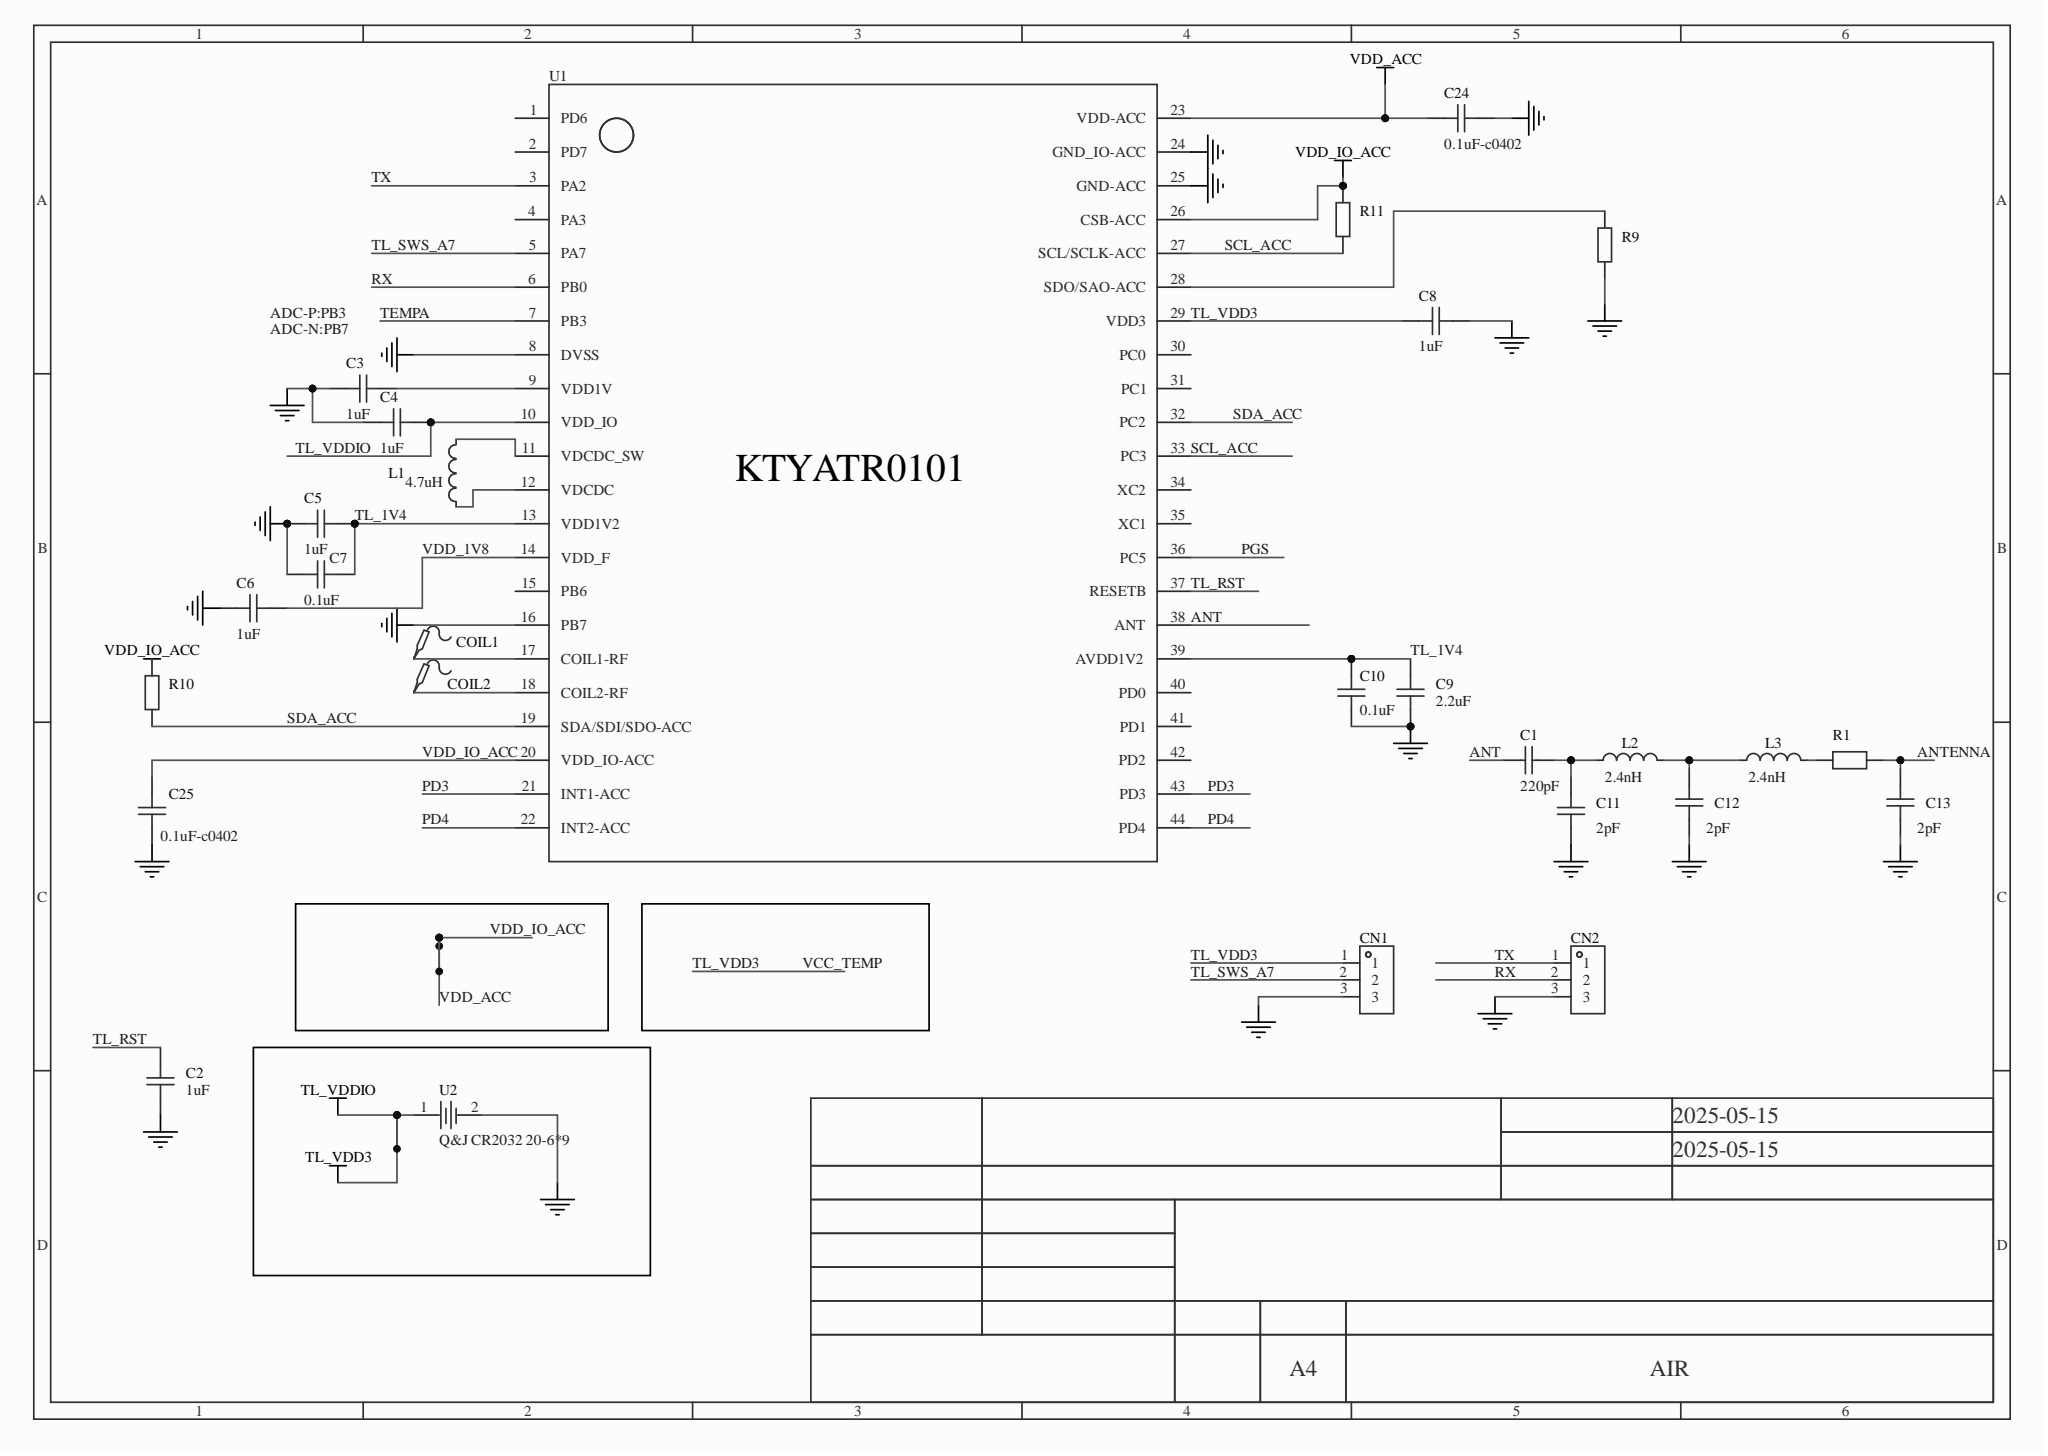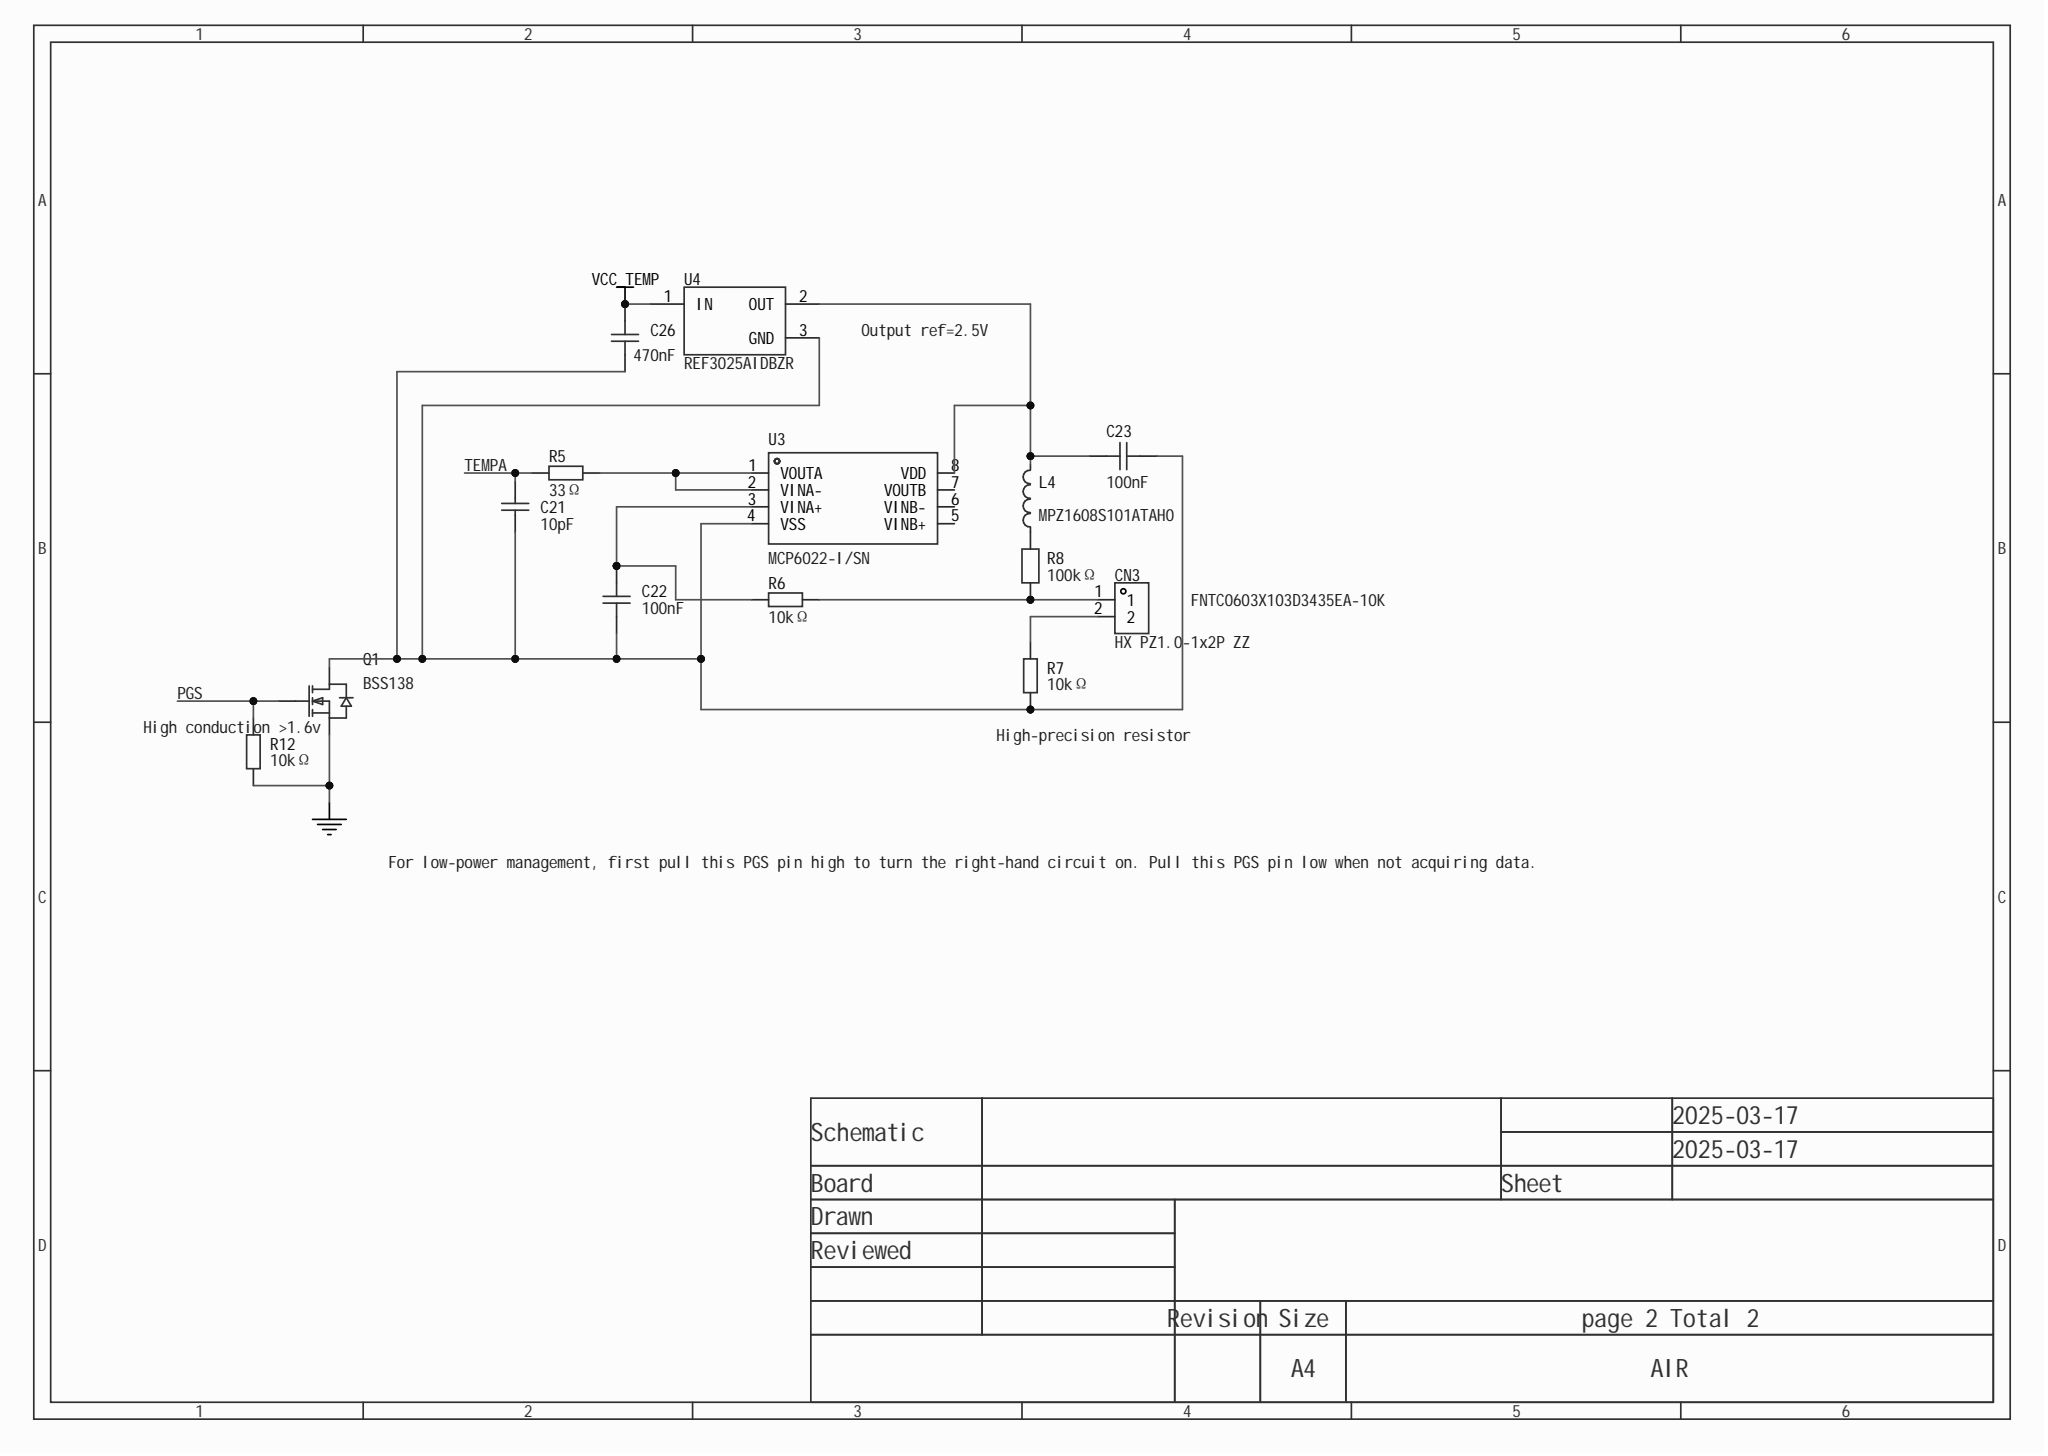Circuit board | Altium Designer | 42 parts | 33 nets
Bill of materials:
Comment,Description,Designator,Footprint,LibRef,Quantity
"220pF","","C1","C0402","CC0402KRX7R9BB221","1"
"1uF","","C2, C3, C4, C5, C6, C8","C0402","CL05A105KA5NQNC","6"
"0.1uF","","C7","C0603","CAP_0603","1"
"2.2uF","","C9","C0402","CL05A105KA5NQNC","1"
"0.1uF","","C10","C0402","CL05A105KA5NQNC","1"
"2pF","","C11, C12, C13","C0402","CC0402CRNPO9BN2R0","3"
"10pF","","C21","C0402","CC0402JRNPO9BN100","1"
"100nF","","C22, C23","C0402","GRM155R71H104KE14D","2"
"0.1uF-c0402","","C24, C25","C0402","0.1uF-c0402","2"
"470nF","","C26","C0402","CGA0402X7R474K100GT","1"
"","","CN1, CN2","HDR-TH_3P-P1.27-V-M-A","3Pin_1.27___","2"
"HX PZ1.0-1x2P ZZ","","CN3","HDR-TH_2P-P1.00-V-M","HX PZ1.0-1x2P ZZ","1"
"","","COIL1, COIL2","Test-Point-0.5mm","Test-Point","2"
"4.7uH","","L1","IND-SMD_L1.8-W1.2","SLC1608F4R7KTT","1"
"2.4nH","","L2, L3","L0402","LQG15HH2N4S02D","2"
"MPZ1608S101ATAH0","","L4","L0603","MPZ1608S101ATAH0","1"
"BSS138","","Q1","SOT-23-3_L3.0-W1.7-P0.95-LS2.9-BR","BSS138","1"
"","","R1, R9, R10, R11","R0402","SCR0402J0R, 0402WGF4701TCE","4"
"33Ω","","R5","R0402","RC0402FR-0733RL","1"
"10kΩ","","R6, R7, R12","R0402","RT0402BRD0710KL, 0402WGF1002TCE","3"
"100kΩ","","R8","R0402","RT0402BRD07100KL","1"
"","","U1","KTYATR0101","KTYATR0101","1"
"Q&J CR2032 20-6*9","","U2","BAT-TH_CR2032","Q&J CR2032 20-6*9","1"
"MCP6022-I/SN","","U3","SOIC-8_L4.9-W3.9-P1.27-LS6.0-BL","MCP6022-I/SN","1"
"REF3025AIDBZR","","U4","SOT-23-3_L2.9-W1.6-P1.90-LS2.8-BR","REF3025AIDBZR","1"
Netlist (Protel format):
[
C1
C0402
220pF



]
[
C2
C0402
1uF



]
[
C3
C0402
1uF



]
[
C4
C0402
1uF



]
[
C5
C0402
1uF



]
[
C6
C0402
1uF



]
[
C7
C0603
0.1uF



]
[
C8
C0402
1uF



]
[
C9
C0402
2.2uF



]
[
C10
C0402
0.1uF



]
[
C11
C0402
2pF



]
[
C12
C0402
2pF



]
[
C13
C0402
2pF



]
[
C21
C0402
10pF



]
[
C22
C0402
100nF



]
[
C23
C0402
100nF



]
[
C24
C0402
0.1uF-c0402



]
[
C25
C0402
0.1uF-c0402



]
[
C26
C0402
470nF



]
[
CN1
HDR-TH_3P-P1.27-V-M-A




]
[
CN2
HDR-TH_3P-P1.27-V-M-A




]
[
CN3
HDR-TH_2P-P1.00-V-M
HX PZ1.0-1x2P ZZ



]
[
COIL1
Test-Point-0.5mm




]
[
COIL2
Test-Point-0.5mm




]
[
L1
IND-SMD_L1.8-W1.2
4.7uH



]
[
L2
L0402
2.4nH



]
[
L3
L0402
2.4nH



]
[
L4
L0603
MPZ1608S101ATAH0



]
[
Q1
SOT-23-3_L3.0-W1.7-P0.95-LS2.9-BR
BSS138



]
[
R1
R0402




]
[
R5
R0402
33Ω



]
[
R6
R0402
10kΩ



]
[
R7
R0402
10kΩ



]
[
R8
R0402
100kΩ



]
[
R9
R0402




]
[
R10
R0402




]
[
R11
R0402




]
[
R12
R0402
10kΩ



]
[
U1
KTYATR0101




]
[
U2
BAT-TH_CR2032
Q&J CR2032 20-6*9



]
[
U3
SOIC-8_L4.9-W3.9-P1.27-LS6.0-BL
MCP6022-I/SN



]
[
U4
SOT-23-3_L2.9-W1.6-P1.90-LS2.8-BR
REF3025AIDBZR



]
(
VDD_ACC
C24-1
C25-1
R10-2
R11-2
U1-20
U1-23
U1-26
)
(
VDD_1V8
C6-2
U1-14
)
(
TX
CN2-1
U1-3
)
(
TL_VDD3
C4-2
C8-1
C26-2
CN1-1
U1-10
U1-29
U2-1
U4-1
)
(
TL_SWS_A7
CN1-2
U1-5
)
(
TL_RST
C2-2
U1-37
)
(
TL_1V4
C5-2
C7-2
C9-2
C10-2
U1-13
U1-39
)
(
TEMPA
C21-2
R5-1
U1-7
)
(
SDA_ACC
R10-1
U1-19
U1-32
)
(
SCL_ACC
R11-1
U1-27
U1-33
)
(
RX
CN2-2
U1-6
)
(
PGS
Q1-1
R12-2
U1-36
)
(
PD4
U1-22
U1-44
)
(
PD3
U1-21
U1-43
)
(
NetR9_2
R9-2
U1-28
)
(
NetR5_2
R5-2
U3-1
U3-2
)
(
NetL4_1
L4-1
R8-2
)
(
NetL3_2
L3-2
R1-1
)
(
NetL1_2
L1-2
U1-11
)
(
NetL1_1
L1-1
U1-12
)
(
NetCOIL2_1
COIL2-1
U1-18
)
(
NetCOIL1_1
COIL1-1
U1-17
)
(
NetCN3_2
CN3-2
R7-2
)
(
NetCN3_1
CN3-1
R6-1
R8-1
)
(
NetC23_1
C23-1
L4-2
U3-8
U4-2
)
(
NetC22_2
C22-2
R6-2
U3-3
)
(
NetC21_1
C21-1
C22-1
C23-2
C26-1
Q1-3
R7-1
U3-4
U4-3
)
(
NetC12_2
C12-2
L2-2
L3-1
)
(
NetC3_2
C3-2
U1-9
)
(
NetC1_2
C1-2
C11-2
L2-1
)
(
GND
C2-1
C3-1
C4-1
C5-1
C6-1
C7-1
C8-2
C9-1
C10-1
C11-1
C12-1
C13-1
C24-2
C25-2
CN1-3
CN2-3
Q1-2
R9-1
R12-1
U1-8
U1-16
U1-24
U1-25
U2-2
)
(
ANTENNA
C13-2
R1-2
)
(
ANT
C1-1
U1-38
)